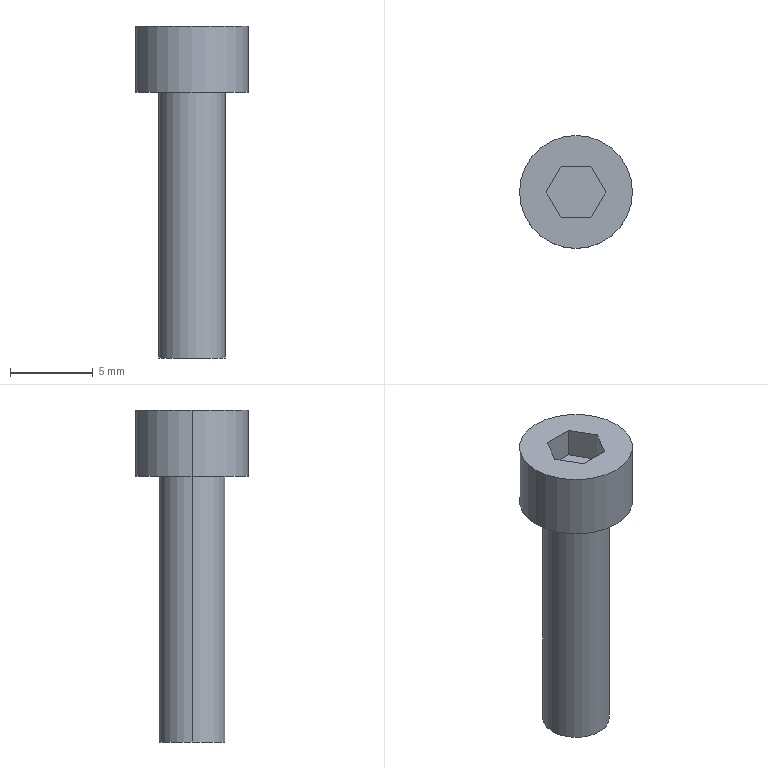Part | SolidWorks | features BaseBody 1 | 1 solid | 14 faces | box 6.8 x 6.8 x 20 mm | volume 331.177 mm3 | plane 10 | cylinder 4 | commonest cylinder face diameters 4 x2 6.8 x2
STEP:
#1=CARTESIAN_POINT('',(2.,0.,-16.));
#2=VERTEX_POINT('',#1);
#3=CARTESIAN_POINT('',(-2.,0.,-16.));
#4=VERTEX_POINT('',#3);
#5=CARTESIAN_POINT('',(0.,0.,-16.));
#6=DIRECTION('',(0.,0.,1.));
#7=DIRECTION('',(1.,0.,0.));
#8=AXIS2_PLACEMENT_3D('',#5,#6,#7);
#9=CIRCLE('',#8,2.);
#10=EDGE_CURVE('',#2,#4,#9,.T.);
#11=ORIENTED_EDGE('',*,*,#10,.T.);
#12=CARTESIAN_POINT('',(-2.,0.,0.));
#13=VERTEX_POINT('',#12);
#14=CARTESIAN_POINT('',(-2.,0.,-16.));
#15=DIRECTION('',(0.,0.,1.));
#16=VECTOR('',#15,1000.);
#17=LINE('',#14,#16);
#18=EDGE_CURVE('',#4,#13,#17,.T.);
#19=ORIENTED_EDGE('',*,*,#18,.T.);
#20=CARTESIAN_POINT('',(2.,0.,0.));
#21=VERTEX_POINT('',#20);
#22=CARTESIAN_POINT('',(0.,0.,0.));
#23=DIRECTION('',(0.,0.,-1.));
#24=DIRECTION('',(1.,0.,0.));
#25=AXIS2_PLACEMENT_3D('',#22,#23,#24);
#26=CIRCLE('',#25,2.);
#27=EDGE_CURVE('',#13,#21,#26,.T.);
#28=ORIENTED_EDGE('',*,*,#27,.T.);
#29=CARTESIAN_POINT('',(2.,0.,-16.));
#30=DIRECTION('',(0.,0.,1.));
#31=VECTOR('',#30,1000.);
#32=LINE('',#29,#31);
#33=EDGE_CURVE('',#2,#21,#32,.T.);
#34=ORIENTED_EDGE('',*,*,#33,.F.);
#35=EDGE_LOOP('',(#11,#19,#28,#34));
#36=FACE_OUTER_BOUND('',#35,.T.);
#37=CARTESIAN_POINT('',(0.,0.,-16.));
#38=DIRECTION('',(0.,0.,1.));
#39=DIRECTION('',(1.,0.,0.));
#40=AXIS2_PLACEMENT_3D('',#37,#38,#39);
#41=CYLINDRICAL_SURFACE('',#40,2.);
#42=ADVANCED_FACE('',(#36),#41,.T.);
#43=CARTESIAN_POINT('',(3.4,0.,0.));
#44=VERTEX_POINT('',#43);
#45=CARTESIAN_POINT('',(-3.4,0.,0.));
#46=VERTEX_POINT('',#45);
#47=CARTESIAN_POINT('',(0.,0.,0.));
#48=DIRECTION('',(0.,0.,1.));
#49=DIRECTION('',(1.,0.,0.));
#50=AXIS2_PLACEMENT_3D('',#47,#48,#49);
#51=CIRCLE('',#50,3.4);
#52=EDGE_CURVE('',#44,#46,#51,.T.);
#53=ORIENTED_EDGE('',*,*,#52,.T.);
#54=CARTESIAN_POINT('',(-3.4,0.,4.));
#55=VERTEX_POINT('',#54);
#56=CARTESIAN_POINT('',(-3.4,0.,0.));
#57=DIRECTION('',(0.,0.,1.));
#58=VECTOR('',#57,1000.);
#59=LINE('',#56,#58);
#60=EDGE_CURVE('',#46,#55,#59,.T.);
#61=ORIENTED_EDGE('',*,*,#60,.T.);
#62=CARTESIAN_POINT('',(3.4,0.,4.));
#63=VERTEX_POINT('',#62);
#64=CARTESIAN_POINT('',(0.,0.,4.));
#65=DIRECTION('',(0.,0.,-1.));
#66=DIRECTION('',(1.,0.,0.));
#67=AXIS2_PLACEMENT_3D('',#64,#65,#66);
#68=CIRCLE('',#67,3.4);
#69=EDGE_CURVE('',#55,#63,#68,.T.);
#70=ORIENTED_EDGE('',*,*,#69,.T.);
#71=CARTESIAN_POINT('',(3.4,0.,0.));
#72=DIRECTION('',(0.,0.,1.));
#73=VECTOR('',#72,1000.);
#74=LINE('',#71,#73);
#75=EDGE_CURVE('',#44,#63,#74,.T.);
#76=ORIENTED_EDGE('',*,*,#75,.F.);
#77=EDGE_LOOP('',(#53,#61,#70,#76));
#78=FACE_OUTER_BOUND('',#77,.T.);
#79=CARTESIAN_POINT('',(0.,0.,0.));
#80=DIRECTION('',(0.,0.,1.));
#81=DIRECTION('',(1.,0.,0.));
#82=AXIS2_PLACEMENT_3D('',#79,#80,#81);
#83=CYLINDRICAL_SURFACE('',#82,3.4);
#84=ADVANCED_FACE('',(#78),#83,.T.);
#85=ORIENTED_EDGE('',*,*,#18,.F.);
#86=CARTESIAN_POINT('',(0.,0.,-16.));
#87=DIRECTION('',(0.,0.,1.));
#88=DIRECTION('',(1.,0.,0.));
#89=AXIS2_PLACEMENT_3D('',#86,#87,#88);
#90=CIRCLE('',#89,2.);
#91=EDGE_CURVE('',#4,#2,#90,.T.);
#92=ORIENTED_EDGE('',*,*,#91,.T.);
#93=ORIENTED_EDGE('',*,*,#33,.T.);
#94=CARTESIAN_POINT('',(0.,0.,0.));
#95=DIRECTION('',(0.,0.,-1.));
#96=DIRECTION('',(1.,0.,0.));
#97=AXIS2_PLACEMENT_3D('',#94,#95,#96);
#98=CIRCLE('',#97,2.);
#99=EDGE_CURVE('',#21,#13,#98,.T.);
#100=ORIENTED_EDGE('',*,*,#99,.T.);
#101=EDGE_LOOP('',(#85,#92,#93,#100));
#102=FACE_OUTER_BOUND('',#101,.T.);
#103=CARTESIAN_POINT('',(0.,0.,-16.));
#104=DIRECTION('',(0.,0.,1.));
#105=DIRECTION('',(1.,0.,0.));
#106=AXIS2_PLACEMENT_3D('',#103,#104,#105);
#107=CYLINDRICAL_SURFACE('',#106,2.);
#108=ADVANCED_FACE('',(#102),#107,.T.);
#109=ORIENTED_EDGE('',*,*,#10,.F.);
#110=ORIENTED_EDGE('',*,*,#91,.F.);
#111=EDGE_LOOP('',(#109,#110));
#112=FACE_OUTER_BOUND('',#111,.T.);
#113=CARTESIAN_POINT('',(0.,0.,-16.));
#114=DIRECTION('',(0.,0.,1.));
#115=DIRECTION('',(1.,0.,0.));
#116=AXIS2_PLACEMENT_3D('',#113,#114,#115);
#117=PLANE('',#116);
#118=ADVANCED_FACE('',(#112),#117,.F.);
#119=ORIENTED_EDGE('',*,*,#99,.F.);
#120=ORIENTED_EDGE('',*,*,#27,.F.);
#121=EDGE_LOOP('',(#119,#120));
#122=FACE_BOUND('',#121,.T.);
#123=ORIENTED_EDGE('',*,*,#52,.F.);
#124=CARTESIAN_POINT('',(0.,0.,0.));
#125=DIRECTION('',(0.,0.,1.));
#126=DIRECTION('',(1.,0.,0.));
#127=AXIS2_PLACEMENT_3D('',#124,#125,#126);
#128=CIRCLE('',#127,3.4);
#129=EDGE_CURVE('',#46,#44,#128,.T.);
#130=ORIENTED_EDGE('',*,*,#129,.F.);
#131=EDGE_LOOP('',(#123,#130));
#132=FACE_OUTER_BOUND('',#131,.T.);
#133=CARTESIAN_POINT('',(0.,0.,0.));
#134=DIRECTION('',(0.,0.,1.));
#135=DIRECTION('',(1.,0.,0.));
#136=AXIS2_PLACEMENT_3D('',#133,#134,#135);
#137=PLANE('',#136);
#138=ADVANCED_FACE('',(#122,#132),#137,.F.);
#139=ORIENTED_EDGE('',*,*,#60,.F.);
#140=ORIENTED_EDGE('',*,*,#129,.T.);
#141=ORIENTED_EDGE('',*,*,#75,.T.);
#142=CARTESIAN_POINT('',(0.,0.,4.));
#143=DIRECTION('',(0.,0.,-1.));
#144=DIRECTION('',(1.,0.,0.));
#145=AXIS2_PLACEMENT_3D('',#142,#143,#144);
#146=CIRCLE('',#145,3.4);
#147=EDGE_CURVE('',#63,#55,#146,.T.);
#148=ORIENTED_EDGE('',*,*,#147,.T.);
#149=EDGE_LOOP('',(#139,#140,#141,#148));
#150=FACE_OUTER_BOUND('',#149,.T.);
#151=CARTESIAN_POINT('',(0.,0.,0.));
#152=DIRECTION('',(0.,0.,1.));
#153=DIRECTION('',(1.,0.,0.));
#154=AXIS2_PLACEMENT_3D('',#151,#152,#153);
#155=CYLINDRICAL_SURFACE('',#154,3.4);
#156=ADVANCED_FACE('',(#150),#155,.T.);
#157=CARTESIAN_POINT('',(-0.9,-1.559,4.));
#158=VERTEX_POINT('',#157);
#159=CARTESIAN_POINT('',(-1.8,0.,4.));
#160=VERTEX_POINT('',#159);
#161=CARTESIAN_POINT('',(-0.9,-1.559,4.));
#162=DIRECTION('',(-0.5,0.866,0.));
#163=VECTOR('',#162,1000.);
#164=LINE('',#161,#163);
#165=EDGE_CURVE('',#158,#160,#164,.T.);
#166=ORIENTED_EDGE('',*,*,#165,.T.);
#167=CARTESIAN_POINT('',(-0.9,1.559,4.));
#168=VERTEX_POINT('',#167);
#169=CARTESIAN_POINT('',(-1.8,0.,4.));
#170=DIRECTION('',(0.5,0.866,0.));
#171=VECTOR('',#170,1000.);
#172=LINE('',#169,#171);
#173=EDGE_CURVE('',#160,#168,#172,.T.);
#174=ORIENTED_EDGE('',*,*,#173,.T.);
#175=CARTESIAN_POINT('',(0.9,1.559,4.));
#176=VERTEX_POINT('',#175);
#177=CARTESIAN_POINT('',(0.,1.559,4.));
#178=DIRECTION('',(1.,0.,0.));
#179=VECTOR('',#178,1000.);
#180=LINE('',#177,#179);
#181=EDGE_CURVE('',#168,#176,#180,.T.);
#182=ORIENTED_EDGE('',*,*,#181,.T.);
#183=CARTESIAN_POINT('',(1.8,0.,4.));
#184=VERTEX_POINT('',#183);
#185=CARTESIAN_POINT('',(0.9,1.559,4.));
#186=DIRECTION('',(0.5,-0.866,0.));
#187=VECTOR('',#186,1000.);
#188=LINE('',#185,#187);
#189=EDGE_CURVE('',#176,#184,#188,.T.);
#190=ORIENTED_EDGE('',*,*,#189,.T.);
#191=CARTESIAN_POINT('',(0.9,-1.559,4.));
#192=VERTEX_POINT('',#191);
#193=CARTESIAN_POINT('',(1.8,0.,4.));
#194=DIRECTION('',(-0.5,-0.866,0.));
#195=VECTOR('',#194,1000.);
#196=LINE('',#193,#195);
#197=EDGE_CURVE('',#184,#192,#196,.T.);
#198=ORIENTED_EDGE('',*,*,#197,.T.);
#199=CARTESIAN_POINT('',(0.,-1.559,4.));
#200=DIRECTION('',(-1.,0.,0.));
#201=VECTOR('',#200,1000.);
#202=LINE('',#199,#201);
#203=EDGE_CURVE('',#192,#158,#202,.T.);
#204=ORIENTED_EDGE('',*,*,#203,.T.);
#205=EDGE_LOOP('',(#166,#174,#182,#190,#198,#204));
#206=FACE_BOUND('',#205,.T.);
#207=ORIENTED_EDGE('',*,*,#147,.F.);
#208=ORIENTED_EDGE('',*,*,#69,.F.);
#209=EDGE_LOOP('',(#207,#208));
#210=FACE_OUTER_BOUND('',#209,.T.);
#211=CARTESIAN_POINT('',(0.,0.,4.));
#212=DIRECTION('',(0.,0.,1.));
#213=DIRECTION('',(1.,0.,0.));
#214=AXIS2_PLACEMENT_3D('',#211,#212,#213);
#215=PLANE('',#214);
#216=ADVANCED_FACE('',(#206,#210),#215,.T.);
#217=ORIENTED_EDGE('',*,*,#173,.F.);
#218=CARTESIAN_POINT('',(-1.8,0.,2.2));
#219=VERTEX_POINT('',#218);
#220=CARTESIAN_POINT('',(-1.8,0.,2.2));
#221=DIRECTION('',(0.,0.,-1.));
#222=VECTOR('',#221,1000.);
#223=LINE('',#220,#222);
#224=EDGE_CURVE('',#160,#219,#223,.T.);
#225=ORIENTED_EDGE('',*,*,#224,.T.);
#226=CARTESIAN_POINT('',(-0.9,1.559,2.2));
#227=VERTEX_POINT('',#226);
#228=CARTESIAN_POINT('',(-0.9,1.559,2.2));
#229=DIRECTION('',(0.5,0.866,0.));
#230=VECTOR('',#229,1000.);
#231=LINE('',#228,#230);
#232=EDGE_CURVE('',#219,#227,#231,.T.);
#233=ORIENTED_EDGE('',*,*,#232,.T.);
#234=CARTESIAN_POINT('',(-0.9,1.559,2.2));
#235=DIRECTION('',(0.,0.,1.));
#236=VECTOR('',#235,1000.);
#237=LINE('',#234,#236);
#238=EDGE_CURVE('',#227,#168,#237,.T.);
#239=ORIENTED_EDGE('',*,*,#238,.T.);
#240=EDGE_LOOP('',(#217,#225,#233,#239));
#241=FACE_OUTER_BOUND('',#240,.T.);
#242=CARTESIAN_POINT('',(-0.9,1.559,2.2));
#243=DIRECTION('',(0.866,-0.5,0.));
#244=DIRECTION('',(0.5,0.866,0.));
#245=AXIS2_PLACEMENT_3D('',#242,#243,#244);
#246=PLANE('',#245);
#247=ADVANCED_FACE('',(#241),#246,.T.);
#248=ORIENTED_EDGE('',*,*,#165,.F.);
#249=CARTESIAN_POINT('',(-0.9,-1.559,2.2));
#250=VERTEX_POINT('',#249);
#251=CARTESIAN_POINT('',(-0.9,-1.559,2.2));
#252=DIRECTION('',(0.,0.,-1.));
#253=VECTOR('',#252,1000.);
#254=LINE('',#251,#253);
#255=EDGE_CURVE('',#158,#250,#254,.T.);
#256=ORIENTED_EDGE('',*,*,#255,.T.);
#257=CARTESIAN_POINT('',(-1.8,0.,2.2));
#258=DIRECTION('',(-0.5,0.866,0.));
#259=VECTOR('',#258,1000.);
#260=LINE('',#257,#259);
#261=EDGE_CURVE('',#250,#219,#260,.T.);
#262=ORIENTED_EDGE('',*,*,#261,.T.);
#263=ORIENTED_EDGE('',*,*,#224,.F.);
#264=EDGE_LOOP('',(#248,#256,#262,#263));
#265=FACE_OUTER_BOUND('',#264,.T.);
#266=CARTESIAN_POINT('',(-1.8,0.,2.2));
#267=DIRECTION('',(0.866,0.5,0.));
#268=DIRECTION('',(-0.5,0.866,0.));
#269=AXIS2_PLACEMENT_3D('',#266,#267,#268);
#270=PLANE('',#269);
#271=ADVANCED_FACE('',(#265),#270,.T.);
#272=ORIENTED_EDGE('',*,*,#203,.F.);
#273=CARTESIAN_POINT('',(0.9,-1.559,2.2));
#274=VERTEX_POINT('',#273);
#275=CARTESIAN_POINT('',(0.9,-1.559,2.2));
#276=DIRECTION('',(0.,0.,-1.));
#277=VECTOR('',#276,1000.);
#278=LINE('',#275,#277);
#279=EDGE_CURVE('',#192,#274,#278,.T.);
#280=ORIENTED_EDGE('',*,*,#279,.T.);
#281=CARTESIAN_POINT('',(-0.9,-1.559,2.2));
#282=DIRECTION('',(-1.,0.,0.));
#283=VECTOR('',#282,1000.);
#284=LINE('',#281,#283);
#285=EDGE_CURVE('',#274,#250,#284,.T.);
#286=ORIENTED_EDGE('',*,*,#285,.T.);
#287=ORIENTED_EDGE('',*,*,#255,.F.);
#288=EDGE_LOOP('',(#272,#280,#286,#287));
#289=FACE_OUTER_BOUND('',#288,.T.);
#290=CARTESIAN_POINT('',(-0.9,-1.559,2.2));
#291=DIRECTION('',(0.,1.,0.));
#292=DIRECTION('',(-1.,0.,0.));
#293=AXIS2_PLACEMENT_3D('',#290,#291,#292);
#294=PLANE('',#293);
#295=ADVANCED_FACE('',(#289),#294,.T.);
#296=ORIENTED_EDGE('',*,*,#197,.F.);
#297=CARTESIAN_POINT('',(1.8,0.,2.2));
#298=VERTEX_POINT('',#297);
#299=CARTESIAN_POINT('',(1.8,0.,2.2));
#300=DIRECTION('',(0.,0.,-1.));
#301=VECTOR('',#300,1000.);
#302=LINE('',#299,#301);
#303=EDGE_CURVE('',#184,#298,#302,.T.);
#304=ORIENTED_EDGE('',*,*,#303,.T.);
#305=CARTESIAN_POINT('',(0.9,-1.559,2.2));
#306=DIRECTION('',(-0.5,-0.866,0.));
#307=VECTOR('',#306,1000.);
#308=LINE('',#305,#307);
#309=EDGE_CURVE('',#298,#274,#308,.T.);
#310=ORIENTED_EDGE('',*,*,#309,.T.);
#311=ORIENTED_EDGE('',*,*,#279,.F.);
#312=EDGE_LOOP('',(#296,#304,#310,#311));
#313=FACE_OUTER_BOUND('',#312,.T.);
#314=CARTESIAN_POINT('',(0.9,-1.559,2.2));
#315=DIRECTION('',(-0.866,0.5,0.));
#316=DIRECTION('',(-0.5,-0.866,0.));
#317=AXIS2_PLACEMENT_3D('',#314,#315,#316);
#318=PLANE('',#317);
#319=ADVANCED_FACE('',(#313),#318,.T.);
#320=ORIENTED_EDGE('',*,*,#189,.F.);
#321=CARTESIAN_POINT('',(0.9,1.559,2.2));
#322=VERTEX_POINT('',#321);
#323=CARTESIAN_POINT('',(0.9,1.559,2.2));
#324=DIRECTION('',(0.,0.,-1.));
#325=VECTOR('',#324,1000.);
#326=LINE('',#323,#325);
#327=EDGE_CURVE('',#176,#322,#326,.T.);
#328=ORIENTED_EDGE('',*,*,#327,.T.);
#329=CARTESIAN_POINT('',(1.8,0.,2.2));
#330=DIRECTION('',(0.5,-0.866,0.));
#331=VECTOR('',#330,1000.);
#332=LINE('',#329,#331);
#333=EDGE_CURVE('',#322,#298,#332,.T.);
#334=ORIENTED_EDGE('',*,*,#333,.T.);
#335=ORIENTED_EDGE('',*,*,#303,.F.);
#336=EDGE_LOOP('',(#320,#328,#334,#335));
#337=FACE_OUTER_BOUND('',#336,.T.);
#338=CARTESIAN_POINT('',(1.8,0.,2.2));
#339=DIRECTION('',(-0.866,-0.5,0.));
#340=DIRECTION('',(0.5,-0.866,0.));
#341=AXIS2_PLACEMENT_3D('',#338,#339,#340);
#342=PLANE('',#341);
#343=ADVANCED_FACE('',(#337),#342,.T.);
#344=ORIENTED_EDGE('',*,*,#181,.F.);
#345=ORIENTED_EDGE('',*,*,#238,.F.);
#346=CARTESIAN_POINT('',(0.9,1.559,2.2));
#347=DIRECTION('',(1.,0.,0.));
#348=VECTOR('',#347,1000.);
#349=LINE('',#346,#348);
#350=EDGE_CURVE('',#227,#322,#349,.T.);
#351=ORIENTED_EDGE('',*,*,#350,.T.);
#352=ORIENTED_EDGE('',*,*,#327,.F.);
#353=EDGE_LOOP('',(#344,#345,#351,#352));
#354=FACE_OUTER_BOUND('',#353,.T.);
#355=CARTESIAN_POINT('',(0.9,1.559,2.2));
#356=DIRECTION('',(0.,-1.,0.));
#357=DIRECTION('',(1.,0.,0.));
#358=AXIS2_PLACEMENT_3D('',#355,#356,#357);
#359=PLANE('',#358);
#360=ADVANCED_FACE('',(#354),#359,.T.);
#361=ORIENTED_EDGE('',*,*,#285,.F.);
#362=ORIENTED_EDGE('',*,*,#309,.F.);
#363=ORIENTED_EDGE('',*,*,#333,.F.);
#364=ORIENTED_EDGE('',*,*,#350,.F.);
#365=ORIENTED_EDGE('',*,*,#232,.F.);
#366=ORIENTED_EDGE('',*,*,#261,.F.);
#367=EDGE_LOOP('',(#361,#362,#363,#364,#365,#366));
#368=FACE_OUTER_BOUND('',#367,.T.);
#369=CARTESIAN_POINT('',(0.,0.,2.2));
#370=DIRECTION('',(0.,0.,1.));
#371=DIRECTION('',(1.,0.,0.));
#372=AXIS2_PLACEMENT_3D('',#369,#370,#371);
#373=PLANE('',#372);
#374=ADVANCED_FACE('',(#368),#373,.T.);
#375=CLOSED_SHELL('',(#42,#84,#108,#118,#138,#156,#216,#247,#271,#295,#319,#343,#360,#374));
#376=MANIFOLD_SOLID_BREP('',#375);
#377=CARTESIAN_POINT('',(0.,0.,0.));
#378=DIRECTION('',(0.,0.,1.));
#379=DIRECTION('',(1.,0.,0.));
#380=AXIS2_PLACEMENT_3D('',#377,#378,#379);
#381=(LENGTH_UNIT()NAMED_UNIT(*)SI_UNIT(.MILLI.,.METRE.));
#382=UNCERTAINTY_MEASURE_WITH_UNIT(LENGTH_MEASURE(0.00001),#381,'','');
#383=(NAMED_UNIT(*)PLANE_ANGLE_UNIT()SI_UNIT($,.RADIAN.));
#384=(NAMED_UNIT(*)SI_UNIT($,.STERADIAN.)SOLID_ANGLE_UNIT());
#385=(GEOMETRIC_REPRESENTATION_CONTEXT(3)GLOBAL_UNCERTAINTY_ASSIGNED_CONTEXT((#382))GLOBAL_UNIT_ASSIGNED_CONTEXT((#381,#383,#384))REPRESENTATION_CONTEXT('',''));
#386=ADVANCED_BREP_SHAPE_REPRESENTATION('',(#376,#380),#385);